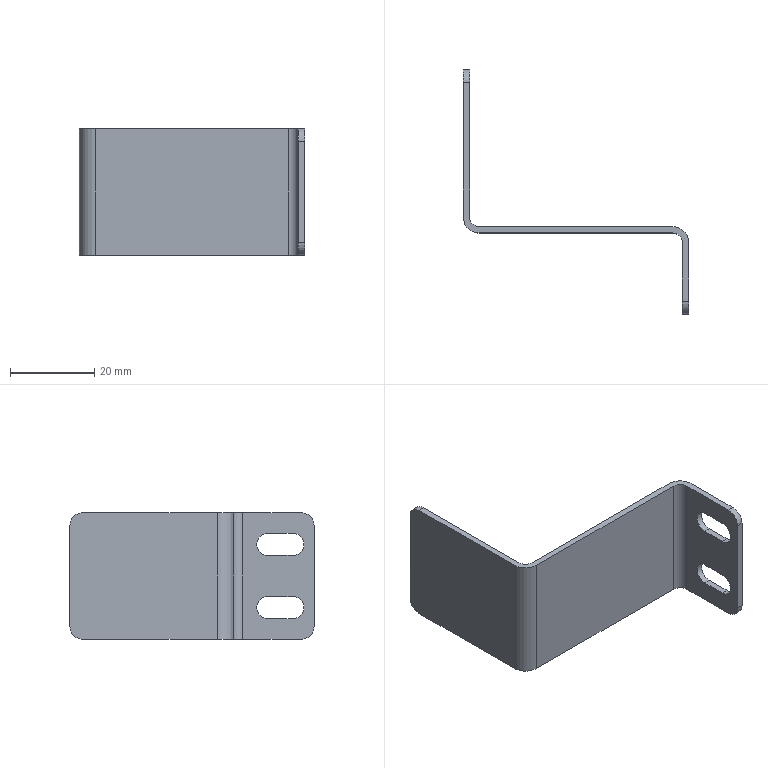Part | SolidWorks | features ExtruThin 1, Fillet 1, ICE 1 | 1 solid | 26 faces | box 53.5 x 58 x 30 mm | volume 4665 mm3 | plane 14 | cylinder 12 | commonest cylinder face diameters 5.2 x4 6 x4 4.5 x2 7.5 x2
STEP:
#1=CARTESIAN_POINT('',(-51.25,23.,0.));
#2=VERTEX_POINT('',#1);
#3=CARTESIAN_POINT('',(-51.25,55.,0.));
#4=VERTEX_POINT('',#3);
#5=CARTESIAN_POINT('',(-51.25,23.,0.));
#6=DIRECTION('',(0.,1.,0.));
#7=VECTOR('',#6,1000.);
#8=LINE('',#5,#7);
#9=EDGE_CURVE('',#2,#4,#8,.T.);
#10=ORIENTED_EDGE('',*,*,#9,.T.);
#11=CARTESIAN_POINT('',(-51.25,58.,3.));
#12=VERTEX_POINT('',#11);
#13=CARTESIAN_POINT('',(-51.25,55.,3.));
#14=DIRECTION('',(1.,0.,0.));
#15=DIRECTION('',(0.,0.,1.));
#16=AXIS2_PLACEMENT_3D('',#13,#14,#15);
#17=CIRCLE('',#16,3.);
#18=EDGE_CURVE('',#4,#12,#17,.T.);
#19=ORIENTED_EDGE('',*,*,#18,.T.);
#20=CARTESIAN_POINT('',(-51.25,58.,27.));
#21=VERTEX_POINT('',#20);
#22=CARTESIAN_POINT('',(-51.25,58.,30.));
#23=DIRECTION('',(0.,0.,-1.));
#24=VECTOR('',#23,1000.);
#25=LINE('',#22,#24);
#26=EDGE_CURVE('',#21,#12,#25,.T.);
#27=ORIENTED_EDGE('',*,*,#26,.F.);
#28=CARTESIAN_POINT('',(-51.25,55.,30.));
#29=VERTEX_POINT('',#28);
#30=CARTESIAN_POINT('',(-51.25,55.,27.));
#31=DIRECTION('',(1.,0.,0.));
#32=DIRECTION('',(0.,0.,1.));
#33=AXIS2_PLACEMENT_3D('',#30,#31,#32);
#34=CIRCLE('',#33,3.);
#35=EDGE_CURVE('',#21,#29,#34,.T.);
#36=ORIENTED_EDGE('',*,*,#35,.T.);
#37=CARTESIAN_POINT('',(-51.25,23.,30.));
#38=VERTEX_POINT('',#37);
#39=CARTESIAN_POINT('',(-51.25,23.,30.));
#40=DIRECTION('',(0.,1.,0.));
#41=VECTOR('',#40,1000.);
#42=LINE('',#39,#41);
#43=EDGE_CURVE('',#38,#29,#42,.T.);
#44=ORIENTED_EDGE('',*,*,#43,.F.);
#45=CARTESIAN_POINT('',(-51.25,23.,30.));
#46=DIRECTION('',(0.,0.,-1.));
#47=VECTOR('',#46,1000.);
#48=LINE('',#45,#47);
#49=EDGE_CURVE('',#38,#2,#48,.T.);
#50=ORIENTED_EDGE('',*,*,#49,.T.);
#51=EDGE_LOOP('',(#10,#19,#27,#36,#44,#50));
#52=FACE_OUTER_BOUND('',#51,.T.);
#53=CARTESIAN_POINT('',(-51.25,23.,30.));
#54=DIRECTION('',(-1.,0.,0.));
#55=DIRECTION('',(0.,0.,1.));
#56=AXIS2_PLACEMENT_3D('',#53,#54,#55);
#57=PLANE('',#56);
#58=ADVANCED_FACE('',(#52),#57,.F.);
#59=ORIENTED_EDGE('',*,*,#26,.T.);
#60=CARTESIAN_POINT('',(-52.75,58.,3.));
#61=VERTEX_POINT('',#60);
#62=CARTESIAN_POINT('',(-52.75,58.,3.));
#63=DIRECTION('',(-1.,0.,0.));
#64=VECTOR('',#63,1000.);
#65=LINE('',#62,#64);
#66=EDGE_CURVE('',#12,#61,#65,.T.);
#67=ORIENTED_EDGE('',*,*,#66,.T.);
#68=CARTESIAN_POINT('',(-52.75,58.,27.));
#69=VERTEX_POINT('',#68);
#70=CARTESIAN_POINT('',(-52.75,58.,30.));
#71=DIRECTION('',(0.,0.,-1.));
#72=VECTOR('',#71,1000.);
#73=LINE('',#70,#72);
#74=EDGE_CURVE('',#69,#61,#73,.T.);
#75=ORIENTED_EDGE('',*,*,#74,.F.);
#76=CARTESIAN_POINT('',(-52.75,58.,27.));
#77=DIRECTION('',(1.,0.,0.));
#78=VECTOR('',#77,1000.);
#79=LINE('',#76,#78);
#80=EDGE_CURVE('',#69,#21,#79,.T.);
#81=ORIENTED_EDGE('',*,*,#80,.T.);
#82=EDGE_LOOP('',(#59,#67,#75,#81));
#83=FACE_OUTER_BOUND('',#82,.T.);
#84=CARTESIAN_POINT('',(-52.75,58.,30.));
#85=DIRECTION('',(0.,1.,0.));
#86=DIRECTION('',(0.,0.,1.));
#87=AXIS2_PLACEMENT_3D('',#84,#85,#86);
#88=PLANE('',#87);
#89=ADVANCED_FACE('',(#83),#88,.T.);
#90=ORIENTED_EDGE('',*,*,#74,.T.);
#91=CARTESIAN_POINT('',(-52.75,55.,0.));
#92=VERTEX_POINT('',#91);
#93=CARTESIAN_POINT('',(-52.75,55.,3.));
#94=DIRECTION('',(-1.,0.,0.));
#95=DIRECTION('',(0.,0.,1.));
#96=AXIS2_PLACEMENT_3D('',#93,#94,#95);
#97=CIRCLE('',#96,3.);
#98=EDGE_CURVE('',#61,#92,#97,.T.);
#99=ORIENTED_EDGE('',*,*,#98,.T.);
#100=CARTESIAN_POINT('',(-52.75,23.,0.));
#101=VERTEX_POINT('',#100);
#102=CARTESIAN_POINT('',(-52.75,23.,0.));
#103=DIRECTION('',(0.,1.,0.));
#104=VECTOR('',#103,1000.);
#105=LINE('',#102,#104);
#106=EDGE_CURVE('',#101,#92,#105,.T.);
#107=ORIENTED_EDGE('',*,*,#106,.F.);
#108=CARTESIAN_POINT('',(-52.75,23.,30.));
#109=VERTEX_POINT('',#108);
#110=CARTESIAN_POINT('',(-52.75,23.,30.));
#111=DIRECTION('',(0.,0.,-1.));
#112=VECTOR('',#111,1000.);
#113=LINE('',#110,#112);
#114=EDGE_CURVE('',#109,#101,#113,.T.);
#115=ORIENTED_EDGE('',*,*,#114,.F.);
#116=CARTESIAN_POINT('',(-52.75,55.,30.));
#117=VERTEX_POINT('',#116);
#118=CARTESIAN_POINT('',(-52.75,23.,30.));
#119=DIRECTION('',(0.,1.,0.));
#120=VECTOR('',#119,1000.);
#121=LINE('',#118,#120);
#122=EDGE_CURVE('',#109,#117,#121,.T.);
#123=ORIENTED_EDGE('',*,*,#122,.T.);
#124=CARTESIAN_POINT('',(-52.75,55.,27.));
#125=DIRECTION('',(-1.,0.,0.));
#126=DIRECTION('',(0.,0.,1.));
#127=AXIS2_PLACEMENT_3D('',#124,#125,#126);
#128=CIRCLE('',#127,3.);
#129=EDGE_CURVE('',#117,#69,#128,.T.);
#130=ORIENTED_EDGE('',*,*,#129,.T.);
#131=EDGE_LOOP('',(#90,#99,#107,#115,#123,#130));
#132=FACE_OUTER_BOUND('',#131,.T.);
#133=CARTESIAN_POINT('',(-52.75,23.,30.));
#134=DIRECTION('',(-1.,0.,0.));
#135=DIRECTION('',(0.,0.,1.));
#136=AXIS2_PLACEMENT_3D('',#133,#134,#135);
#137=PLANE('',#136);
#138=ADVANCED_FACE('',(#132),#137,.T.);
#139=CARTESIAN_POINT('',(-49.,19.25,0.));
#140=VERTEX_POINT('',#139);
#141=CARTESIAN_POINT('',(-49.,23.,0.));
#142=DIRECTION('',(0.,0.,-1.));
#143=DIRECTION('',(1.,0.,0.));
#144=AXIS2_PLACEMENT_3D('',#141,#142,#143);
#145=CIRCLE('',#144,3.75);
#146=EDGE_CURVE('',#140,#101,#145,.T.);
#147=ORIENTED_EDGE('',*,*,#146,.F.);
#148=CARTESIAN_POINT('',(-49.,19.25,30.));
#149=VERTEX_POINT('',#148);
#150=CARTESIAN_POINT('',(-49.,19.25,30.));
#151=DIRECTION('',(0.,0.,-1.));
#152=VECTOR('',#151,1000.);
#153=LINE('',#150,#152);
#154=EDGE_CURVE('',#149,#140,#153,.T.);
#155=ORIENTED_EDGE('',*,*,#154,.F.);
#156=CARTESIAN_POINT('',(-49.,23.,30.));
#157=DIRECTION('',(0.,0.,-1.));
#158=DIRECTION('',(1.,0.,0.));
#159=AXIS2_PLACEMENT_3D('',#156,#157,#158);
#160=CIRCLE('',#159,3.75);
#161=EDGE_CURVE('',#149,#109,#160,.T.);
#162=ORIENTED_EDGE('',*,*,#161,.T.);
#163=ORIENTED_EDGE('',*,*,#114,.T.);
#164=EDGE_LOOP('',(#147,#155,#162,#163));
#165=FACE_OUTER_BOUND('',#164,.T.);
#166=CARTESIAN_POINT('',(-49.,23.,30.));
#167=DIRECTION('',(0.,0.,-1.));
#168=DIRECTION('',(-1.,0.,0.));
#169=AXIS2_PLACEMENT_3D('',#166,#167,#168);
#170=CYLINDRICAL_SURFACE('',#169,3.75);
#171=ADVANCED_FACE('',(#165),#170,.T.);
#172=CARTESIAN_POINT('',(-3.,19.25,0.));
#173=VERTEX_POINT('',#172);
#174=CARTESIAN_POINT('',(-3.,19.25,0.));
#175=DIRECTION('',(-1.,0.,0.));
#176=VECTOR('',#175,1000.);
#177=LINE('',#174,#176);
#178=EDGE_CURVE('',#173,#140,#177,.T.);
#179=ORIENTED_EDGE('',*,*,#178,.F.);
#180=CARTESIAN_POINT('',(-3.,19.25,30.));
#181=VERTEX_POINT('',#180);
#182=CARTESIAN_POINT('',(-3.,19.25,30.));
#183=DIRECTION('',(0.,0.,-1.));
#184=VECTOR('',#183,1000.);
#185=LINE('',#182,#184);
#186=EDGE_CURVE('',#181,#173,#185,.T.);
#187=ORIENTED_EDGE('',*,*,#186,.F.);
#188=CARTESIAN_POINT('',(-3.,19.25,30.));
#189=DIRECTION('',(-1.,0.,0.));
#190=VECTOR('',#189,1000.);
#191=LINE('',#188,#190);
#192=EDGE_CURVE('',#181,#149,#191,.T.);
#193=ORIENTED_EDGE('',*,*,#192,.T.);
#194=ORIENTED_EDGE('',*,*,#154,.T.);
#195=EDGE_LOOP('',(#179,#187,#193,#194));
#196=FACE_OUTER_BOUND('',#195,.T.);
#197=CARTESIAN_POINT('',(-3.,19.25,30.));
#198=DIRECTION('',(0.,-1.,0.));
#199=DIRECTION('',(1.,0.,0.));
#200=AXIS2_PLACEMENT_3D('',#197,#198,#199);
#201=PLANE('',#200);
#202=ADVANCED_FACE('',(#196),#201,.T.);
#203=CARTESIAN_POINT('',(-0.75,17.,0.));
#204=VERTEX_POINT('',#203);
#205=CARTESIAN_POINT('',(-3.,17.,0.));
#206=DIRECTION('',(0.,0.,1.));
#207=DIRECTION('',(1.,0.,0.));
#208=AXIS2_PLACEMENT_3D('',#205,#206,#207);
#209=CIRCLE('',#208,2.25);
#210=EDGE_CURVE('',#204,#173,#209,.T.);
#211=ORIENTED_EDGE('',*,*,#210,.F.);
#212=CARTESIAN_POINT('',(-0.75,17.,30.));
#213=VERTEX_POINT('',#212);
#214=CARTESIAN_POINT('',(-0.75,17.,30.));
#215=DIRECTION('',(0.,0.,-1.));
#216=VECTOR('',#215,1000.);
#217=LINE('',#214,#216);
#218=EDGE_CURVE('',#213,#204,#217,.T.);
#219=ORIENTED_EDGE('',*,*,#218,.F.);
#220=CARTESIAN_POINT('',(-3.,17.,30.));
#221=DIRECTION('',(0.,0.,1.));
#222=DIRECTION('',(1.,0.,0.));
#223=AXIS2_PLACEMENT_3D('',#220,#221,#222);
#224=CIRCLE('',#223,2.25);
#225=EDGE_CURVE('',#213,#181,#224,.T.);
#226=ORIENTED_EDGE('',*,*,#225,.T.);
#227=ORIENTED_EDGE('',*,*,#186,.T.);
#228=EDGE_LOOP('',(#211,#219,#226,#227));
#229=FACE_OUTER_BOUND('',#228,.T.);
#230=CARTESIAN_POINT('',(-3.,17.,30.));
#231=DIRECTION('',(0.,0.,-1.));
#232=DIRECTION('',(-1.,0.,0.));
#233=AXIS2_PLACEMENT_3D('',#230,#231,#232);
#234=CYLINDRICAL_SURFACE('',#233,2.25);
#235=ADVANCED_FACE('',(#229),#234,.F.);
#236=CARTESIAN_POINT('',(-0.75,11.,10.1));
#237=VERTEX_POINT('',#236);
#238=CARTESIAN_POINT('',(-0.75,11.,4.9));
#239=VERTEX_POINT('',#238);
#240=CARTESIAN_POINT('',(-0.75,11.,7.5));
#241=DIRECTION('',(-1.,0.,0.));
#242=DIRECTION('',(0.,0.,1.));
#243=AXIS2_PLACEMENT_3D('',#240,#241,#242);
#244=CIRCLE('',#243,2.6);
#245=EDGE_CURVE('',#237,#239,#244,.T.);
#246=ORIENTED_EDGE('',*,*,#245,.F.);
#247=CARTESIAN_POINT('',(-0.75,5.,10.1));
#248=VERTEX_POINT('',#247);
#249=CARTESIAN_POINT('',(-0.75,11.,10.1));
#250=DIRECTION('',(0.,1.,0.));
#251=VECTOR('',#250,1000.);
#252=LINE('',#249,#251);
#253=EDGE_CURVE('',#248,#237,#252,.T.);
#254=ORIENTED_EDGE('',*,*,#253,.F.);
#255=CARTESIAN_POINT('',(-0.75,5.,4.9));
#256=VERTEX_POINT('',#255);
#257=CARTESIAN_POINT('',(-0.75,5.,7.5));
#258=DIRECTION('',(-1.,0.,0.));
#259=DIRECTION('',(0.,0.,1.));
#260=AXIS2_PLACEMENT_3D('',#257,#258,#259);
#261=CIRCLE('',#260,2.6);
#262=EDGE_CURVE('',#256,#248,#261,.T.);
#263=ORIENTED_EDGE('',*,*,#262,.F.);
#264=CARTESIAN_POINT('',(-0.75,11.,4.9));
#265=DIRECTION('',(0.,-1.,0.));
#266=VECTOR('',#265,1000.);
#267=LINE('',#264,#266);
#268=EDGE_CURVE('',#239,#256,#267,.T.);
#269=ORIENTED_EDGE('',*,*,#268,.F.);
#270=EDGE_LOOP('',(#246,#254,#263,#269));
#271=FACE_BOUND('',#270,.T.);
#272=CARTESIAN_POINT('',(-0.75,11.,25.1));
#273=VERTEX_POINT('',#272);
#274=CARTESIAN_POINT('',(-0.75,11.,19.9));
#275=VERTEX_POINT('',#274);
#276=CARTESIAN_POINT('',(-0.75,11.,22.5));
#277=DIRECTION('',(-1.,0.,0.));
#278=DIRECTION('',(0.,0.,1.));
#279=AXIS2_PLACEMENT_3D('',#276,#277,#278);
#280=CIRCLE('',#279,2.6);
#281=EDGE_CURVE('',#273,#275,#280,.T.);
#282=ORIENTED_EDGE('',*,*,#281,.F.);
#283=CARTESIAN_POINT('',(-0.75,5.,25.1));
#284=VERTEX_POINT('',#283);
#285=CARTESIAN_POINT('',(-0.75,11.,25.1));
#286=DIRECTION('',(0.,1.,0.));
#287=VECTOR('',#286,1000.);
#288=LINE('',#285,#287);
#289=EDGE_CURVE('',#284,#273,#288,.T.);
#290=ORIENTED_EDGE('',*,*,#289,.F.);
#291=CARTESIAN_POINT('',(-0.75,5.,19.9));
#292=VERTEX_POINT('',#291);
#293=CARTESIAN_POINT('',(-0.75,5.,22.5));
#294=DIRECTION('',(-1.,0.,0.));
#295=DIRECTION('',(0.,0.,1.));
#296=AXIS2_PLACEMENT_3D('',#293,#294,#295);
#297=CIRCLE('',#296,2.6);
#298=EDGE_CURVE('',#292,#284,#297,.T.);
#299=ORIENTED_EDGE('',*,*,#298,.F.);
#300=CARTESIAN_POINT('',(-0.75,11.,19.9));
#301=DIRECTION('',(0.,-1.,0.));
#302=VECTOR('',#301,1000.);
#303=LINE('',#300,#302);
#304=EDGE_CURVE('',#275,#292,#303,.T.);
#305=ORIENTED_EDGE('',*,*,#304,.F.);
#306=EDGE_LOOP('',(#282,#290,#299,#305));
#307=FACE_BOUND('',#306,.T.);
#308=CARTESIAN_POINT('',(-0.75,0.,27.));
#309=VERTEX_POINT('',#308);
#310=CARTESIAN_POINT('',(-0.75,0.,3.));
#311=VERTEX_POINT('',#310);
#312=CARTESIAN_POINT('',(-0.75,0.,30.));
#313=DIRECTION('',(0.,0.,-1.));
#314=VECTOR('',#313,1000.);
#315=LINE('',#312,#314);
#316=EDGE_CURVE('',#309,#311,#315,.T.);
#317=ORIENTED_EDGE('',*,*,#316,.F.);
#318=CARTESIAN_POINT('',(-0.75,3.,30.));
#319=VERTEX_POINT('',#318);
#320=CARTESIAN_POINT('',(-0.75,3.,27.));
#321=DIRECTION('',(-1.,0.,0.));
#322=DIRECTION('',(0.,0.,1.));
#323=AXIS2_PLACEMENT_3D('',#320,#321,#322);
#324=CIRCLE('',#323,3.);
#325=EDGE_CURVE('',#309,#319,#324,.T.);
#326=ORIENTED_EDGE('',*,*,#325,.T.);
#327=CARTESIAN_POINT('',(-0.75,0.,30.));
#328=DIRECTION('',(0.,1.,0.));
#329=VECTOR('',#328,1000.);
#330=LINE('',#327,#329);
#331=EDGE_CURVE('',#319,#213,#330,.T.);
#332=ORIENTED_EDGE('',*,*,#331,.T.);
#333=ORIENTED_EDGE('',*,*,#218,.T.);
#334=CARTESIAN_POINT('',(-0.75,3.,0.));
#335=VERTEX_POINT('',#334);
#336=CARTESIAN_POINT('',(-0.75,0.,0.));
#337=DIRECTION('',(0.,1.,0.));
#338=VECTOR('',#337,1000.);
#339=LINE('',#336,#338);
#340=EDGE_CURVE('',#335,#204,#339,.T.);
#341=ORIENTED_EDGE('',*,*,#340,.F.);
#342=CARTESIAN_POINT('',(-0.75,3.,3.));
#343=DIRECTION('',(-1.,0.,0.));
#344=DIRECTION('',(0.,0.,1.));
#345=AXIS2_PLACEMENT_3D('',#342,#343,#344);
#346=CIRCLE('',#345,3.);
#347=EDGE_CURVE('',#335,#311,#346,.T.);
#348=ORIENTED_EDGE('',*,*,#347,.T.);
#349=EDGE_LOOP('',(#317,#326,#332,#333,#341,#348));
#350=FACE_OUTER_BOUND('',#349,.T.);
#351=CARTESIAN_POINT('',(-0.75,0.,30.));
#352=DIRECTION('',(-1.,0.,0.));
#353=DIRECTION('',(0.,0.,1.));
#354=AXIS2_PLACEMENT_3D('',#351,#352,#353);
#355=PLANE('',#354);
#356=ADVANCED_FACE('',(#271,#307,#350),#355,.T.);
#357=CARTESIAN_POINT('',(0.75,0.,27.));
#358=VERTEX_POINT('',#357);
#359=CARTESIAN_POINT('',(0.75,0.,3.));
#360=VERTEX_POINT('',#359);
#361=CARTESIAN_POINT('',(0.75,0.,30.));
#362=DIRECTION('',(0.,0.,-1.));
#363=VECTOR('',#362,1000.);
#364=LINE('',#361,#363);
#365=EDGE_CURVE('',#358,#360,#364,.T.);
#366=ORIENTED_EDGE('',*,*,#365,.F.);
#367=CARTESIAN_POINT('',(0.75,0.,27.));
#368=DIRECTION('',(-1.,0.,0.));
#369=VECTOR('',#368,1000.);
#370=LINE('',#367,#369);
#371=EDGE_CURVE('',#358,#309,#370,.T.);
#372=ORIENTED_EDGE('',*,*,#371,.T.);
#373=ORIENTED_EDGE('',*,*,#316,.T.);
#374=CARTESIAN_POINT('',(0.75,0.,3.));
#375=DIRECTION('',(1.,0.,0.));
#376=VECTOR('',#375,1000.);
#377=LINE('',#374,#376);
#378=EDGE_CURVE('',#311,#360,#377,.T.);
#379=ORIENTED_EDGE('',*,*,#378,.T.);
#380=EDGE_LOOP('',(#366,#372,#373,#379));
#381=FACE_OUTER_BOUND('',#380,.T.);
#382=CARTESIAN_POINT('',(0.75,0.,30.));
#383=DIRECTION('',(0.,-1.,0.));
#384=DIRECTION('',(0.,0.,-1.));
#385=AXIS2_PLACEMENT_3D('',#382,#383,#384);
#386=PLANE('',#385);
#387=ADVANCED_FACE('',(#381),#386,.T.);
#388=CARTESIAN_POINT('',(0.75,5.,10.1));
#389=VERTEX_POINT('',#388);
#390=CARTESIAN_POINT('',(0.75,11.,10.1));
#391=VERTEX_POINT('',#390);
#392=CARTESIAN_POINT('',(0.75,0.,10.1));
#393=DIRECTION('',(0.,1.,0.));
#394=VECTOR('',#393,1000.);
#395=LINE('',#392,#394);
#396=EDGE_CURVE('',#389,#391,#395,.T.);
#397=ORIENTED_EDGE('',*,*,#396,.T.);
#398=CARTESIAN_POINT('',(0.75,11.,4.9));
#399=VERTEX_POINT('',#398);
#400=CARTESIAN_POINT('',(0.75,11.,7.5));
#401=DIRECTION('',(-1.,0.,0.));
#402=DIRECTION('',(0.,0.,1.));
#403=AXIS2_PLACEMENT_3D('',#400,#401,#402);
#404=CIRCLE('',#403,2.6);
#405=EDGE_CURVE('',#391,#399,#404,.T.);
#406=ORIENTED_EDGE('',*,*,#405,.T.);
#407=CARTESIAN_POINT('',(0.75,5.,4.9));
#408=VERTEX_POINT('',#407);
#409=CARTESIAN_POINT('',(0.75,0.,4.9));
#410=DIRECTION('',(0.,-1.,0.));
#411=VECTOR('',#410,1000.);
#412=LINE('',#409,#411);
#413=EDGE_CURVE('',#399,#408,#412,.T.);
#414=ORIENTED_EDGE('',*,*,#413,.T.);
#415=CARTESIAN_POINT('',(0.75,5.,7.5));
#416=DIRECTION('',(-1.,0.,0.));
#417=DIRECTION('',(0.,0.,1.));
#418=AXIS2_PLACEMENT_3D('',#415,#416,#417);
#419=CIRCLE('',#418,2.6);
#420=EDGE_CURVE('',#408,#389,#419,.T.);
#421=ORIENTED_EDGE('',*,*,#420,.T.);
#422=EDGE_LOOP('',(#397,#406,#414,#421));
#423=FACE_BOUND('',#422,.T.);
#424=CARTESIAN_POINT('',(0.75,5.,25.1));
#425=VERTEX_POINT('',#424);
#426=CARTESIAN_POINT('',(0.75,11.,25.1));
#427=VERTEX_POINT('',#426);
#428=CARTESIAN_POINT('',(0.75,0.,25.1));
#429=DIRECTION('',(0.,1.,0.));
#430=VECTOR('',#429,1000.);
#431=LINE('',#428,#430);
#432=EDGE_CURVE('',#425,#427,#431,.T.);
#433=ORIENTED_EDGE('',*,*,#432,.T.);
#434=CARTESIAN_POINT('',(0.75,11.,19.9));
#435=VERTEX_POINT('',#434);
#436=CARTESIAN_POINT('',(0.75,11.,22.5));
#437=DIRECTION('',(-1.,0.,0.));
#438=DIRECTION('',(0.,0.,1.));
#439=AXIS2_PLACEMENT_3D('',#436,#437,#438);
#440=CIRCLE('',#439,2.6);
#441=EDGE_CURVE('',#427,#435,#440,.T.);
#442=ORIENTED_EDGE('',*,*,#441,.T.);
#443=CARTESIAN_POINT('',(0.75,5.,19.9));
#444=VERTEX_POINT('',#443);
#445=CARTESIAN_POINT('',(0.75,0.,19.9));
#446=DIRECTION('',(0.,-1.,0.));
#447=VECTOR('',#446,1000.);
#448=LINE('',#445,#447);
#449=EDGE_CURVE('',#435,#444,#448,.T.);
#450=ORIENTED_EDGE('',*,*,#449,.T.);
#451=CARTESIAN_POINT('',(0.75,5.,22.5));
#452=DIRECTION('',(-1.,0.,0.));
#453=DIRECTION('',(0.,0.,1.));
#454=AXIS2_PLACEMENT_3D('',#451,#452,#453);
#455=CIRCLE('',#454,2.6);
#456=EDGE_CURVE('',#444,#425,#455,.T.);
#457=ORIENTED_EDGE('',*,*,#456,.T.);
#458=EDGE_LOOP('',(#433,#442,#450,#457));
#459=FACE_BOUND('',#458,.T.);
#460=CARTESIAN_POINT('',(0.75,3.,30.));
#461=VERTEX_POINT('',#460);
#462=CARTESIAN_POINT('',(0.75,17.,30.));
#463=VERTEX_POINT('',#462);
#464=CARTESIAN_POINT('',(0.75,0.,30.));
#465=DIRECTION('',(0.,1.,0.));
#466=VECTOR('',#465,1000.);
#467=LINE('',#464,#466);
#468=EDGE_CURVE('',#461,#463,#467,.T.);
#469=ORIENTED_EDGE('',*,*,#468,.F.);
#470=CARTESIAN_POINT('',(0.75,3.,27.));
#471=DIRECTION('',(1.,0.,0.));
#472=DIRECTION('',(0.,0.,1.));
#473=AXIS2_PLACEMENT_3D('',#470,#471,#472);
#474=CIRCLE('',#473,3.);
#475=EDGE_CURVE('',#461,#358,#474,.T.);
#476=ORIENTED_EDGE('',*,*,#475,.T.);
#477=ORIENTED_EDGE('',*,*,#365,.T.);
#478=CARTESIAN_POINT('',(0.75,3.,0.));
#479=VERTEX_POINT('',#478);
#480=CARTESIAN_POINT('',(0.75,3.,3.));
#481=DIRECTION('',(1.,0.,0.));
#482=DIRECTION('',(0.,0.,1.));
#483=AXIS2_PLACEMENT_3D('',#480,#481,#482);
#484=CIRCLE('',#483,3.);
#485=EDGE_CURVE('',#360,#479,#484,.T.);
#486=ORIENTED_EDGE('',*,*,#485,.T.);
#487=CARTESIAN_POINT('',(0.75,17.,0.));
#488=VERTEX_POINT('',#487);
#489=CARTESIAN_POINT('',(0.75,0.,0.));
#490=DIRECTION('',(0.,1.,0.));
#491=VECTOR('',#490,1000.);
#492=LINE('',#489,#491);
#493=EDGE_CURVE('',#479,#488,#492,.T.);
#494=ORIENTED_EDGE('',*,*,#493,.T.);
#495=CARTESIAN_POINT('',(0.75,17.,30.));
#496=DIRECTION('',(0.,0.,-1.));
#497=VECTOR('',#496,1000.);
#498=LINE('',#495,#497);
#499=EDGE_CURVE('',#463,#488,#498,.T.);
#500=ORIENTED_EDGE('',*,*,#499,.F.);
#501=EDGE_LOOP('',(#469,#476,#477,#486,#494,#500));
#502=FACE_OUTER_BOUND('',#501,.T.);
#503=CARTESIAN_POINT('',(0.75,0.,30.));
#504=DIRECTION('',(-1.,0.,0.));
#505=DIRECTION('',(0.,0.,1.));
#506=AXIS2_PLACEMENT_3D('',#503,#504,#505);
#507=PLANE('',#506);
#508=ADVANCED_FACE('',(#423,#459,#502),#507,.F.);
#509=CARTESIAN_POINT('',(-3.,20.75,0.));
#510=VERTEX_POINT('',#509);
#511=CARTESIAN_POINT('',(-3.,17.,0.));
#512=DIRECTION('',(0.,0.,1.));
#513=DIRECTION('',(1.,0.,0.));
#514=AXIS2_PLACEMENT_3D('',#511,#512,#513);
#515=CIRCLE('',#514,3.75);
#516=EDGE_CURVE('',#488,#510,#515,.T.);
#517=ORIENTED_EDGE('',*,*,#516,.T.);
#518=CARTESIAN_POINT('',(-3.,20.75,30.));
#519=VERTEX_POINT('',#518);
#520=CARTESIAN_POINT('',(-3.,20.75,30.));
#521=DIRECTION('',(0.,0.,-1.));
#522=VECTOR('',#521,1000.);
#523=LINE('',#520,#522);
#524=EDGE_CURVE('',#519,#510,#523,.T.);
#525=ORIENTED_EDGE('',*,*,#524,.F.);
#526=CARTESIAN_POINT('',(-3.,17.,30.));
#527=DIRECTION('',(0.,0.,1.));
#528=DIRECTION('',(1.,0.,0.));
#529=AXIS2_PLACEMENT_3D('',#526,#527,#528);
#530=CIRCLE('',#529,3.75);
#531=EDGE_CURVE('',#463,#519,#530,.T.);
#532=ORIENTED_EDGE('',*,*,#531,.F.);
#533=ORIENTED_EDGE('',*,*,#499,.T.);
#534=EDGE_LOOP('',(#517,#525,#532,#533));
#535=FACE_OUTER_BOUND('',#534,.T.);
#536=CARTESIAN_POINT('',(-3.,17.,30.));
#537=DIRECTION('',(0.,0.,-1.));
#538=DIRECTION('',(-1.,0.,0.));
#539=AXIS2_PLACEMENT_3D('',#536,#537,#538);
#540=CYLINDRICAL_SURFACE('',#539,3.75);
#541=ADVANCED_FACE('',(#535),#540,.T.);
#542=CARTESIAN_POINT('',(-49.,20.75,0.));
#543=VERTEX_POINT('',#542);
#544=CARTESIAN_POINT('',(-3.,20.75,0.));
#545=DIRECTION('',(-1.,0.,0.));
#546=VECTOR('',#545,1000.);
#547=LINE('',#544,#546);
#548=EDGE_CURVE('',#510,#543,#547,.T.);
#549=ORIENTED_EDGE('',*,*,#548,.T.);
#550=CARTESIAN_POINT('',(-49.,20.75,30.));
#551=VERTEX_POINT('',#550);
#552=CARTESIAN_POINT('',(-49.,20.75,30.));
#553=DIRECTION('',(0.,0.,-1.));
#554=VECTOR('',#553,1000.);
#555=LINE('',#552,#554);
#556=EDGE_CURVE('',#551,#543,#555,.T.);
#557=ORIENTED_EDGE('',*,*,#556,.F.);
#558=CARTESIAN_POINT('',(-3.,20.75,30.));
#559=DIRECTION('',(-1.,0.,0.));
#560=VECTOR('',#559,1000.);
#561=LINE('',#558,#560);
#562=EDGE_CURVE('',#519,#551,#561,.T.);
#563=ORIENTED_EDGE('',*,*,#562,.F.);
#564=ORIENTED_EDGE('',*,*,#524,.T.);
#565=EDGE_LOOP('',(#549,#557,#563,#564));
#566=FACE_OUTER_BOUND('',#565,.T.);
#567=CARTESIAN_POINT('',(-3.,20.75,30.));
#568=DIRECTION('',(0.,-1.,0.));
#569=DIRECTION('',(1.,0.,0.));
#570=AXIS2_PLACEMENT_3D('',#567,#568,#569);
#571=PLANE('',#570);
#572=ADVANCED_FACE('',(#566),#571,.F.);
#573=CARTESIAN_POINT('',(-49.,23.,0.));
#574=DIRECTION('',(0.,0.,-1.));
#575=DIRECTION('',(1.,0.,0.));
#576=AXIS2_PLACEMENT_3D('',#573,#574,#575);
#577=CIRCLE('',#576,2.25);
#578=EDGE_CURVE('',#543,#2,#577,.T.);
#579=ORIENTED_EDGE('',*,*,#578,.T.);
#580=ORIENTED_EDGE('',*,*,#49,.F.);
#581=CARTESIAN_POINT('',(-49.,23.,30.));
#582=DIRECTION('',(0.,0.,-1.));
#583=DIRECTION('',(1.,0.,0.));
#584=AXIS2_PLACEMENT_3D('',#581,#582,#583);
#585=CIRCLE('',#584,2.25);
#586=EDGE_CURVE('',#551,#38,#585,.T.);
#587=ORIENTED_EDGE('',*,*,#586,.F.);
#588=ORIENTED_EDGE('',*,*,#556,.T.);
#589=EDGE_LOOP('',(#579,#580,#587,#588));
#590=FACE_OUTER_BOUND('',#589,.T.);
#591=CARTESIAN_POINT('',(-49.,23.,30.));
#592=DIRECTION('',(0.,0.,-1.));
#593=DIRECTION('',(-1.,0.,0.));
#594=AXIS2_PLACEMENT_3D('',#591,#592,#593);
#595=CYLINDRICAL_SURFACE('',#594,2.25);
#596=ADVANCED_FACE('',(#590),#595,.F.);
#597=ORIENTED_EDGE('',*,*,#43,.T.);
#598=CARTESIAN_POINT('',(-49.,55.,30.));
#599=DIRECTION('',(-1.,0.,0.));
#600=VECTOR('',#599,1000.);
#601=LINE('',#598,#600);
#602=EDGE_CURVE('',#29,#117,#601,.T.);
#603=ORIENTED_EDGE('',*,*,#602,.T.);
#604=ORIENTED_EDGE('',*,*,#122,.F.);
#605=ORIENTED_EDGE('',*,*,#161,.F.);
#606=ORIENTED_EDGE('',*,*,#192,.F.);
#607=ORIENTED_EDGE('',*,*,#225,.F.);
#608=ORIENTED_EDGE('',*,*,#331,.F.);
#609=CARTESIAN_POINT('',(-49.,3.,30.));
#610=DIRECTION('',(1.,0.,0.));
#611=VECTOR('',#610,1000.);
#612=LINE('',#609,#611);
#613=EDGE_CURVE('',#319,#461,#612,.T.);
#614=ORIENTED_EDGE('',*,*,#613,.T.);
#615=ORIENTED_EDGE('',*,*,#468,.T.);
#616=ORIENTED_EDGE('',*,*,#531,.T.);
#617=ORIENTED_EDGE('',*,*,#562,.T.);
#618=ORIENTED_EDGE('',*,*,#586,.T.);
#619=EDGE_LOOP('',(#597,#603,#604,#605,#606,#607,#608,#614,#615,#616,#617,#618));
#620=FACE_OUTER_BOUND('',#619,.T.);
#621=CARTESIAN_POINT('',(-49.,23.,30.));
#622=DIRECTION('',(0.,0.,1.));
#623=DIRECTION('',(1.,0.,0.));
#624=AXIS2_PLACEMENT_3D('',#621,#622,#623);
#625=PLANE('',#624);
#626=ADVANCED_FACE('',(#620),#625,.T.);
#627=ORIENTED_EDGE('',*,*,#106,.T.);
#628=CARTESIAN_POINT('',(-51.25,55.,0.));
#629=DIRECTION('',(1.,0.,0.));
#630=VECTOR('',#629,1000.);
#631=LINE('',#628,#630);
#632=EDGE_CURVE('',#92,#4,#631,.T.);
#633=ORIENTED_EDGE('',*,*,#632,.T.);
#634=ORIENTED_EDGE('',*,*,#9,.F.);
#635=ORIENTED_EDGE('',*,*,#578,.F.);
#636=ORIENTED_EDGE('',*,*,#548,.F.);
#637=ORIENTED_EDGE('',*,*,#516,.F.);
#638=ORIENTED_EDGE('',*,*,#493,.F.);
#639=CARTESIAN_POINT('',(-0.75,3.,0.));
#640=DIRECTION('',(-1.,0.,0.));
#641=VECTOR('',#640,1000.);
#642=LINE('',#639,#641);
#643=EDGE_CURVE('',#479,#335,#642,.T.);
#644=ORIENTED_EDGE('',*,*,#643,.T.);
#645=ORIENTED_EDGE('',*,*,#340,.T.);
#646=ORIENTED_EDGE('',*,*,#210,.T.);
#647=ORIENTED_EDGE('',*,*,#178,.T.);
#648=ORIENTED_EDGE('',*,*,#146,.T.);
#649=EDGE_LOOP('',(#627,#633,#634,#635,#636,#637,#638,#644,#645,#646,#647,#648));
#650=FACE_OUTER_BOUND('',#649,.T.);
#651=CARTESIAN_POINT('',(-49.,23.,0.));
#652=DIRECTION('',(0.,0.,1.));
#653=DIRECTION('',(1.,0.,0.));
#654=AXIS2_PLACEMENT_3D('',#651,#652,#653);
#655=PLANE('',#654);
#656=ADVANCED_FACE('',(#650),#655,.F.);
#657=ORIENTED_EDGE('',*,*,#98,.F.);
#658=ORIENTED_EDGE('',*,*,#66,.F.);
#659=ORIENTED_EDGE('',*,*,#18,.F.);
#660=ORIENTED_EDGE('',*,*,#632,.F.);
#661=EDGE_LOOP('',(#657,#658,#659,#660));
#662=FACE_OUTER_BOUND('',#661,.T.);
#663=CARTESIAN_POINT('',(-49.,55.,3.));
#664=DIRECTION('',(-1.,0.,0.));
#665=DIRECTION('',(0.,0.,1.));
#666=AXIS2_PLACEMENT_3D('',#663,#664,#665);
#667=CYLINDRICAL_SURFACE('',#666,3.);
#668=ADVANCED_FACE('',(#662),#667,.T.);
#669=ORIENTED_EDGE('',*,*,#129,.F.);
#670=ORIENTED_EDGE('',*,*,#602,.F.);
#671=ORIENTED_EDGE('',*,*,#35,.F.);
#672=ORIENTED_EDGE('',*,*,#80,.F.);
#673=EDGE_LOOP('',(#669,#670,#671,#672));
#674=FACE_OUTER_BOUND('',#673,.T.);
#675=CARTESIAN_POINT('',(-52.75,55.,27.));
#676=DIRECTION('',(1.,0.,0.));
#677=DIRECTION('',(0.,0.,-1.));
#678=AXIS2_PLACEMENT_3D('',#675,#676,#677);
#679=CYLINDRICAL_SURFACE('',#678,3.);
#680=ADVANCED_FACE('',(#674),#679,.T.);
#681=ORIENTED_EDGE('',*,*,#475,.F.);
#682=ORIENTED_EDGE('',*,*,#613,.F.);
#683=ORIENTED_EDGE('',*,*,#325,.F.);
#684=ORIENTED_EDGE('',*,*,#371,.F.);
#685=EDGE_LOOP('',(#681,#682,#683,#684));
#686=FACE_OUTER_BOUND('',#685,.T.);
#687=CARTESIAN_POINT('',(0.75,3.,27.));
#688=DIRECTION('',(-1.,0.,0.));
#689=DIRECTION('',(0.,0.,1.));
#690=AXIS2_PLACEMENT_3D('',#687,#688,#689);
#691=CYLINDRICAL_SURFACE('',#690,3.);
#692=ADVANCED_FACE('',(#686),#691,.T.);
#693=ORIENTED_EDGE('',*,*,#485,.F.);
#694=ORIENTED_EDGE('',*,*,#378,.F.);
#695=ORIENTED_EDGE('',*,*,#347,.F.);
#696=ORIENTED_EDGE('',*,*,#643,.F.);
#697=EDGE_LOOP('',(#693,#694,#695,#696));
#698=FACE_OUTER_BOUND('',#697,.T.);
#699=CARTESIAN_POINT('',(-49.,3.,3.));
#700=DIRECTION('',(1.,0.,0.));
#701=DIRECTION('',(0.,0.,-1.));
#702=AXIS2_PLACEMENT_3D('',#699,#700,#701);
#703=CYLINDRICAL_SURFACE('',#702,3.);
#704=ADVANCED_FACE('',(#698),#703,.T.);
#705=CARTESIAN_POINT('',(9.25,11.,25.1));
#706=DIRECTION('',(-1.,0.,0.));
#707=VECTOR('',#706,1000.);
#708=LINE('',#705,#707);
#709=EDGE_CURVE('',#427,#273,#708,.T.);
#710=ORIENTED_EDGE('',*,*,#709,.T.);
#711=ORIENTED_EDGE('',*,*,#281,.T.);
#712=CARTESIAN_POINT('',(9.25,11.,19.9));
#713=DIRECTION('',(-1.,0.,0.));
#714=VECTOR('',#713,1000.);
#715=LINE('',#712,#714);
#716=EDGE_CURVE('',#435,#275,#715,.T.);
#717=ORIENTED_EDGE('',*,*,#716,.F.);
#718=ORIENTED_EDGE('',*,*,#441,.F.);
#719=EDGE_LOOP('',(#710,#711,#717,#718));
#720=FACE_OUTER_BOUND('',#719,.T.);
#721=CARTESIAN_POINT('',(9.25,11.,22.5));
#722=DIRECTION('',(-1.,0.,0.));
#723=DIRECTION('',(0.,0.,1.));
#724=AXIS2_PLACEMENT_3D('',#721,#722,#723);
#725=CYLINDRICAL_SURFACE('',#724,2.6);
#726=ADVANCED_FACE('',(#720),#725,.F.);
#727=CARTESIAN_POINT('',(9.25,5.,25.1));
#728=DIRECTION('',(-1.,0.,0.));
#729=VECTOR('',#728,1000.);
#730=LINE('',#727,#729);
#731=EDGE_CURVE('',#425,#284,#730,.T.);
#732=ORIENTED_EDGE('',*,*,#731,.T.);
#733=ORIENTED_EDGE('',*,*,#289,.T.);
#734=ORIENTED_EDGE('',*,*,#709,.F.);
#735=ORIENTED_EDGE('',*,*,#432,.F.);
#736=EDGE_LOOP('',(#732,#733,#734,#735));
#737=FACE_OUTER_BOUND('',#736,.T.);
#738=CARTESIAN_POINT('',(9.25,11.,25.1));
#739=DIRECTION('',(0.,0.,1.));
#740=DIRECTION('',(0.,-1.,0.));
#741=AXIS2_PLACEMENT_3D('',#738,#739,#740);
#742=PLANE('',#741);
#743=ADVANCED_FACE('',(#737),#742,.F.);
#744=CARTESIAN_POINT('',(9.25,5.,19.9));
#745=DIRECTION('',(-1.,0.,0.));
#746=VECTOR('',#745,1000.);
#747=LINE('',#744,#746);
#748=EDGE_CURVE('',#444,#292,#747,.T.);
#749=ORIENTED_EDGE('',*,*,#748,.T.);
#750=ORIENTED_EDGE('',*,*,#298,.T.);
#751=ORIENTED_EDGE('',*,*,#731,.F.);
#752=ORIENTED_EDGE('',*,*,#456,.F.);
#753=EDGE_LOOP('',(#749,#750,#751,#752));
#754=FACE_OUTER_BOUND('',#753,.T.);
#755=CARTESIAN_POINT('',(9.25,5.,22.5));
#756=DIRECTION('',(-1.,0.,0.));
#757=DIRECTION('',(0.,0.,1.));
#758=AXIS2_PLACEMENT_3D('',#755,#756,#757);
#759=CYLINDRICAL_SURFACE('',#758,2.6);
#760=ADVANCED_FACE('',(#754),#759,.F.);
#761=ORIENTED_EDGE('',*,*,#716,.T.);
#762=ORIENTED_EDGE('',*,*,#304,.T.);
#763=ORIENTED_EDGE('',*,*,#748,.F.);
#764=ORIENTED_EDGE('',*,*,#449,.F.);
#765=EDGE_LOOP('',(#761,#762,#763,#764));
#766=FACE_OUTER_BOUND('',#765,.T.);
#767=CARTESIAN_POINT('',(9.25,11.,19.9));
#768=DIRECTION('',(0.,0.,-1.));
#769=DIRECTION('',(0.,1.,0.));
#770=AXIS2_PLACEMENT_3D('',#767,#768,#769);
#771=PLANE('',#770);
#772=ADVANCED_FACE('',(#766),#771,.F.);
#773=CARTESIAN_POINT('',(9.25,11.,10.1));
#774=DIRECTION('',(-1.,0.,0.));
#775=VECTOR('',#774,1000.);
#776=LINE('',#773,#775);
#777=EDGE_CURVE('',#391,#237,#776,.T.);
#778=ORIENTED_EDGE('',*,*,#777,.T.);
#779=ORIENTED_EDGE('',*,*,#245,.T.);
#780=CARTESIAN_POINT('',(9.25,11.,4.9));
#781=DIRECTION('',(-1.,0.,0.));
#782=VECTOR('',#781,1000.);
#783=LINE('',#780,#782);
#784=EDGE_CURVE('',#399,#239,#783,.T.);
#785=ORIENTED_EDGE('',*,*,#784,.F.);
#786=ORIENTED_EDGE('',*,*,#405,.F.);
#787=EDGE_LOOP('',(#778,#779,#785,#786));
#788=FACE_OUTER_BOUND('',#787,.T.);
#789=CARTESIAN_POINT('',(9.25,11.,7.5));
#790=DIRECTION('',(-1.,0.,0.));
#791=DIRECTION('',(0.,0.,1.));
#792=AXIS2_PLACEMENT_3D('',#789,#790,#791);
#793=CYLINDRICAL_SURFACE('',#792,2.6);
#794=ADVANCED_FACE('',(#788),#793,.F.);
#795=CARTESIAN_POINT('',(9.25,5.,10.1));
#796=DIRECTION('',(-1.,0.,0.));
#797=VECTOR('',#796,1000.);
#798=LINE('',#795,#797);
#799=EDGE_CURVE('',#389,#248,#798,.T.);
#800=ORIENTED_EDGE('',*,*,#799,.T.);
#801=ORIENTED_EDGE('',*,*,#253,.T.);
#802=ORIENTED_EDGE('',*,*,#777,.F.);
#803=ORIENTED_EDGE('',*,*,#396,.F.);
#804=EDGE_LOOP('',(#800,#801,#802,#803));
#805=FACE_OUTER_BOUND('',#804,.T.);
#806=CARTESIAN_POINT('',(9.25,11.,10.1));
#807=DIRECTION('',(0.,0.,1.));
#808=DIRECTION('',(1.,0.,0.));
#809=AXIS2_PLACEMENT_3D('',#806,#807,#808);
#810=PLANE('',#809);
#811=ADVANCED_FACE('',(#805),#810,.F.);
#812=CARTESIAN_POINT('',(9.25,5.,4.9));
#813=DIRECTION('',(-1.,0.,0.));
#814=VECTOR('',#813,1000.);
#815=LINE('',#812,#814);
#816=EDGE_CURVE('',#408,#256,#815,.T.);
#817=ORIENTED_EDGE('',*,*,#816,.T.);
#818=ORIENTED_EDGE('',*,*,#262,.T.);
#819=ORIENTED_EDGE('',*,*,#799,.F.);
#820=ORIENTED_EDGE('',*,*,#420,.F.);
#821=EDGE_LOOP('',(#817,#818,#819,#820));
#822=FACE_OUTER_BOUND('',#821,.T.);
#823=CARTESIAN_POINT('',(9.25,5.,7.5));
#824=DIRECTION('',(-1.,0.,0.));
#825=DIRECTION('',(0.,0.,1.));
#826=AXIS2_PLACEMENT_3D('',#823,#824,#825);
#827=CYLINDRICAL_SURFACE('',#826,2.6);
#828=ADVANCED_FACE('',(#822),#827,.F.);
#829=ORIENTED_EDGE('',*,*,#784,.T.);
#830=ORIENTED_EDGE('',*,*,#268,.T.);
#831=ORIENTED_EDGE('',*,*,#816,.F.);
#832=ORIENTED_EDGE('',*,*,#413,.F.);
#833=EDGE_LOOP('',(#829,#830,#831,#832));
#834=FACE_OUTER_BOUND('',#833,.T.);
#835=CARTESIAN_POINT('',(9.25,11.,4.9));
#836=DIRECTION('',(0.,0.,-1.));
#837=DIRECTION('',(-1.,0.,0.));
#838=AXIS2_PLACEMENT_3D('',#835,#836,#837);
#839=PLANE('',#838);
#840=ADVANCED_FACE('',(#834),#839,.F.);
#841=CLOSED_SHELL('',(#58,#89,#138,#171,#202,#235,#356,#387,#508,#541,#572,#596,#626,#656,#668,#680,#692,#704,#726,#743,#760,#772,#794,#811,#828,#840));
#842=MANIFOLD_SOLID_BREP('',#841);
#843=CARTESIAN_POINT('',(0.,0.,0.));
#844=DIRECTION('',(0.,0.,1.));
#845=DIRECTION('',(1.,0.,0.));
#846=AXIS2_PLACEMENT_3D('',#843,#844,#845);
#847=(LENGTH_UNIT()NAMED_UNIT(*)SI_UNIT(.MILLI.,.METRE.));
#848=UNCERTAINTY_MEASURE_WITH_UNIT(LENGTH_MEASURE(0.00001),#847,'','');
#849=(NAMED_UNIT(*)PLANE_ANGLE_UNIT()SI_UNIT($,.RADIAN.));
#850=(NAMED_UNIT(*)SI_UNIT($,.STERADIAN.)SOLID_ANGLE_UNIT());
#851=(GEOMETRIC_REPRESENTATION_CONTEXT(3)GLOBAL_UNCERTAINTY_ASSIGNED_CONTEXT((#848))GLOBAL_UNIT_ASSIGNED_CONTEXT((#847,#849,#850))REPRESENTATION_CONTEXT('',''));
#852=ADVANCED_BREP_SHAPE_REPRESENTATION('',(#842,#846),#851);